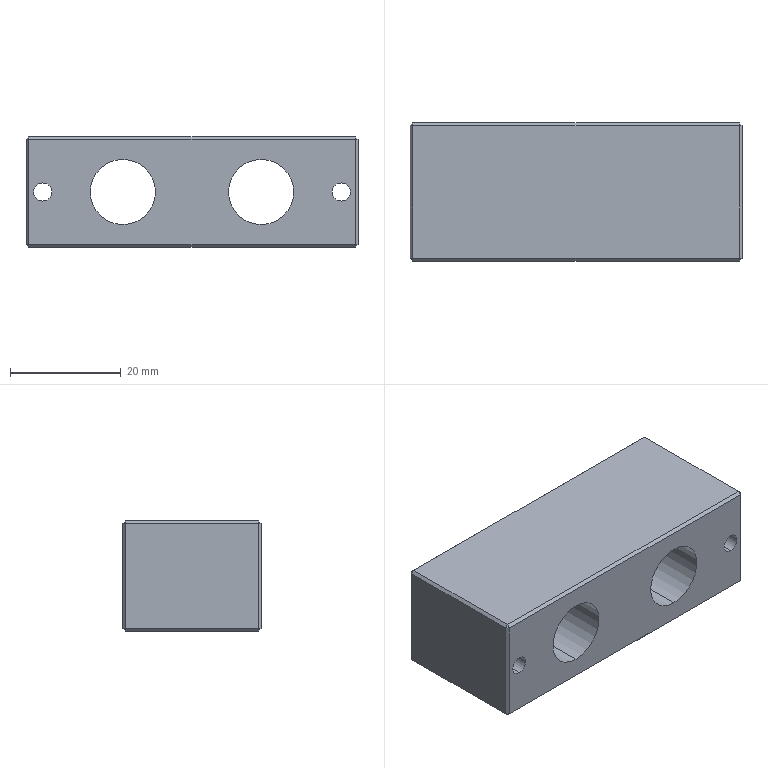Part | STEP file | silencer fixing block | 1 solid | 34 faces | box 60 x 25 x 20 mm | volume 24053 mm3 | plane 26 | cylinder 8 | commonest cylinder face diameters 3.3 x4 11.8 x4